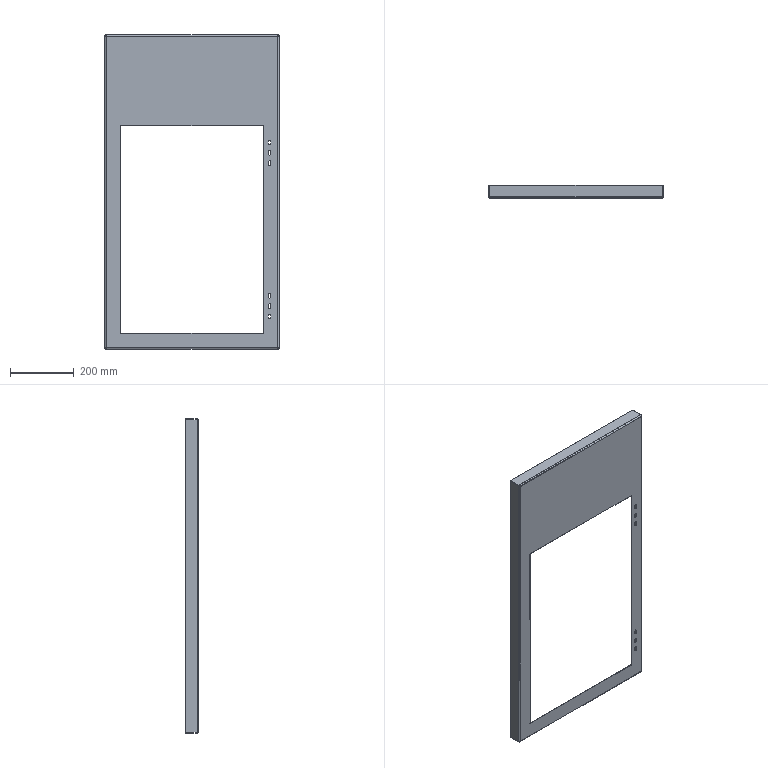Part | SolidWorks | features ICE 2, EdgeFlange 1, FlatPattern 1, SMBaseFlange 1, SheetMetal 1 | 1 solid | 76 faces | box 546 x 40 x 985 mm | volume 712813 mm3 | plane 38 | cylinder 30 | spline 8 | commonest cylinder face diameters 9 x18 4 x8 8 x4